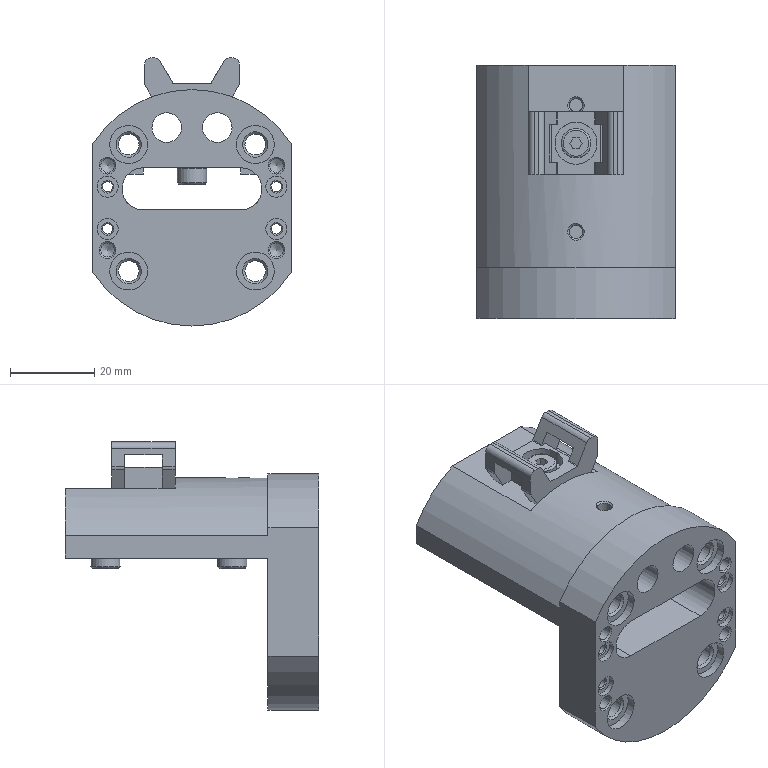Part | STEP file | 540883_HAPG_72_B_2_14b | 5 solids | 199 faces | box 47 x 60 x 63.5 mm | volume 42972 mm3 | plane 91 | cylinder 54 | cone 53 | torus 1 | commonest cylinder face diameters 3 x8 9 x8 3.242 x7 5 x5 7 x5 0.4 x4